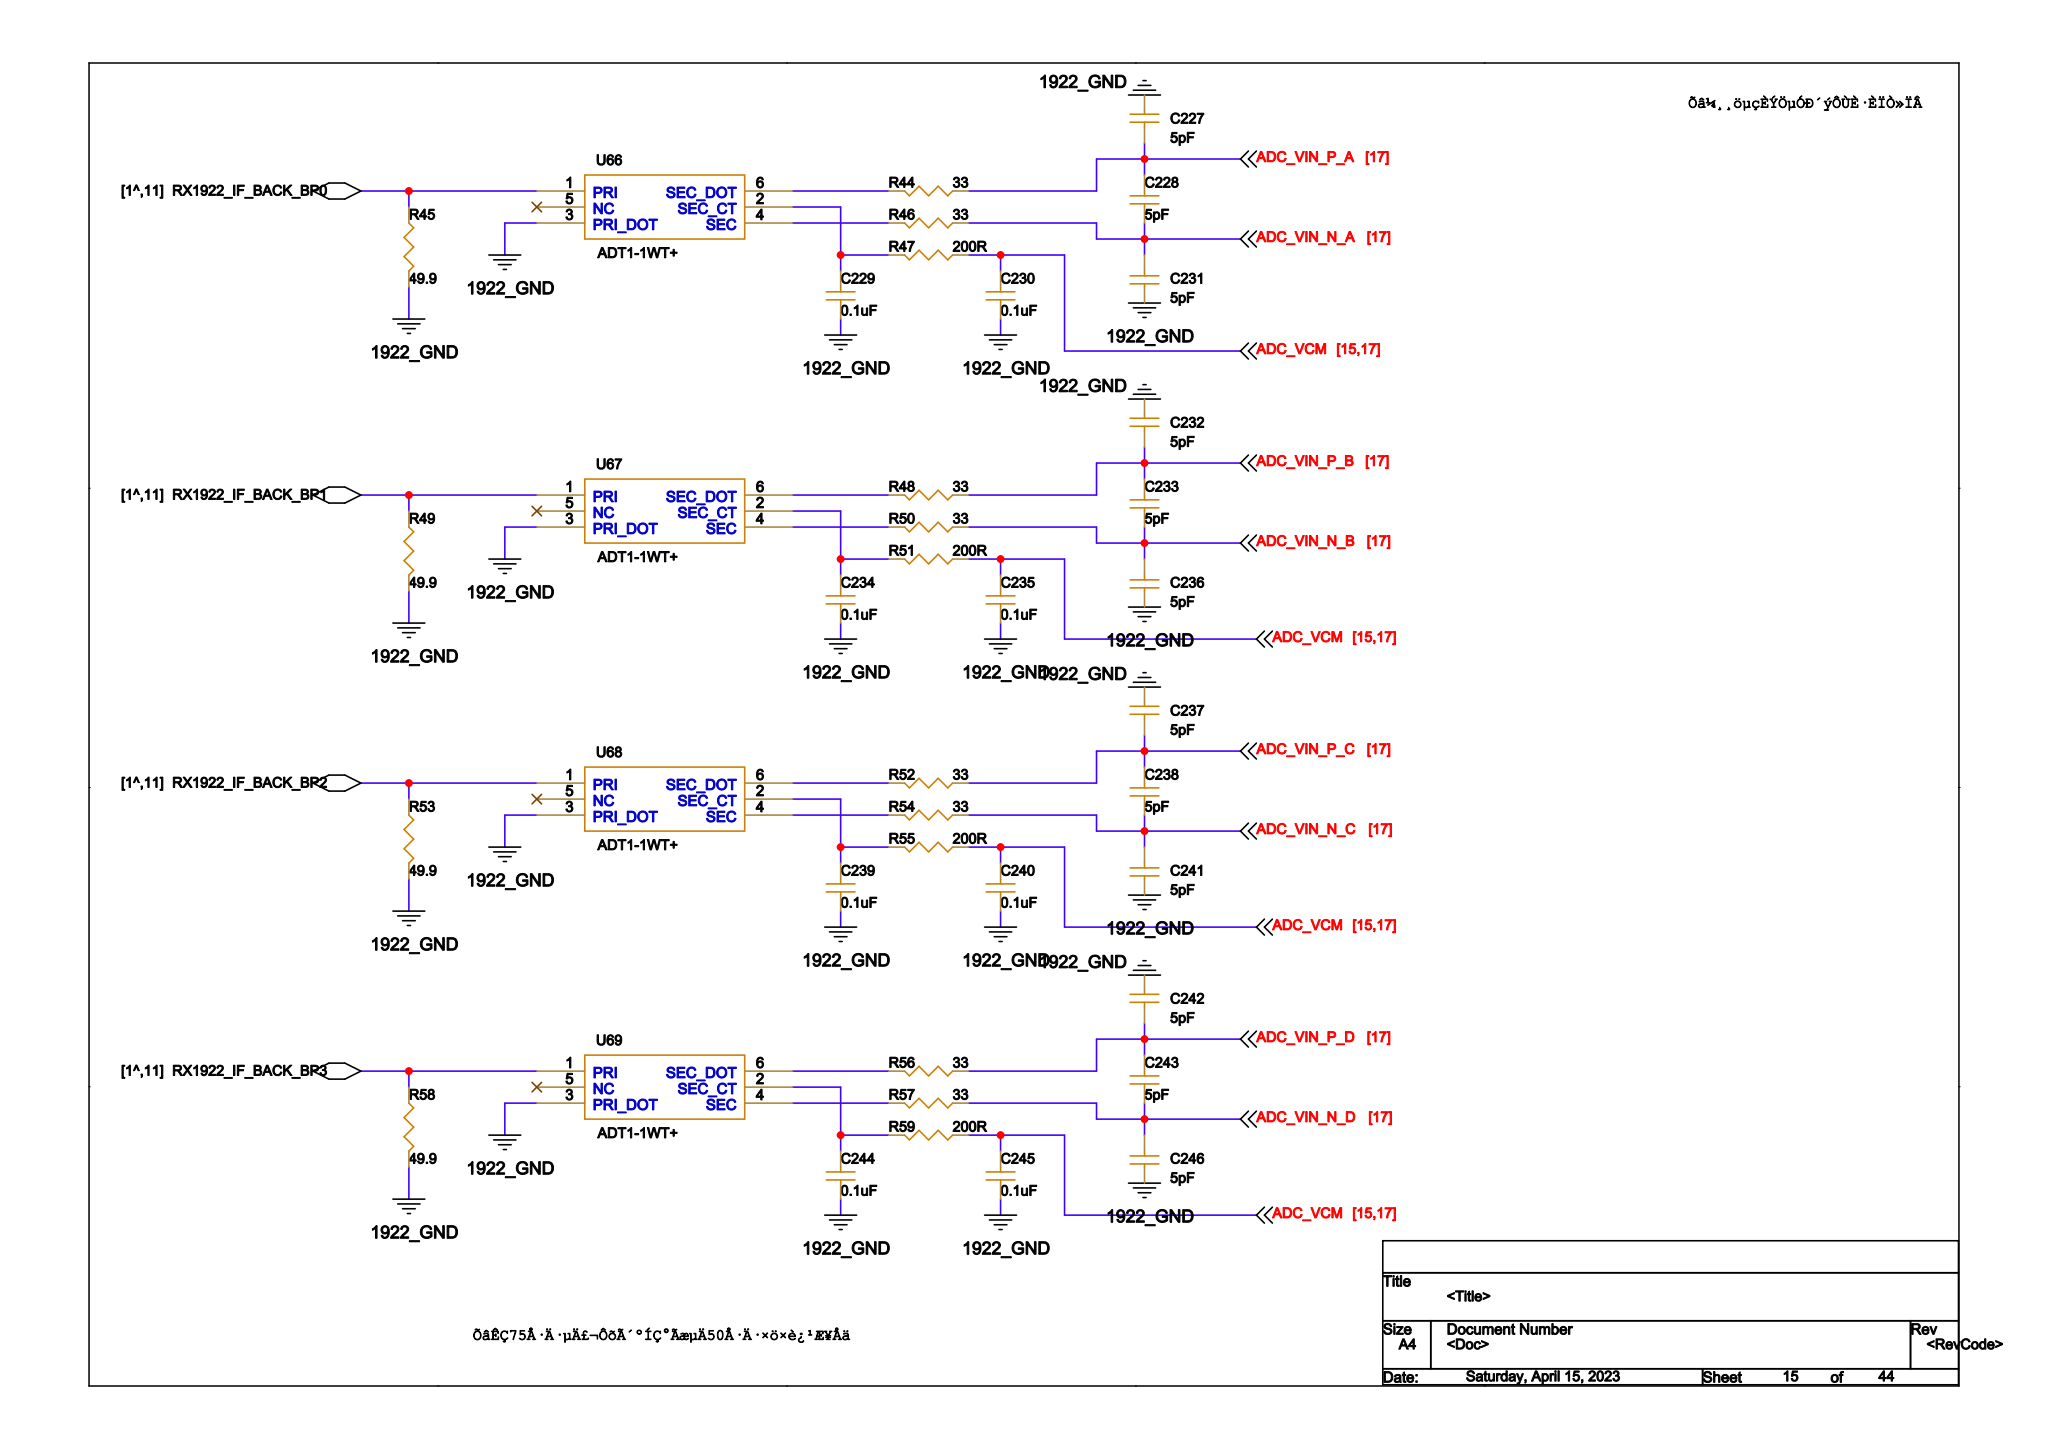Circuit board | Cadence Allegro | 1034 parts | 912 nets | one sheet of the schematic
Parts on this sheet (reference | value | footprint):
C227 | 5pF | C0402
C228 | 5pF | C0402
C229 | 0.1uF | C0402
C230 | 0.1uF | C0402
C231 | 5pF | C0402
C232 | 5pF | C0402
C233 | 5pF | C0402
C234 | 0.1uF | C0402
C235 | 0.1uF | C0402
C236 | 5pF | C0402
C237 | 5pF | C0402
C238 | 5pF | C0402
C239 | 0.1uF | C0402
C240 | 0.1uF | C0402
C241 | 5pF | C0402
C242 | 5pF | C0402
C243 | 5pF | C0402
C244 | 0.1uF | C0402
C245 | 0.1uF | C0402
C246 | 5pF | C0402
R44 | 33 | R0402
R45 | 49.9 | R0402
R46 | 33 | R0402
R47 | 200R | R0402
R48 | 33 | R0402
R49 | 49.9 | R0402
R50 | 33 | R0402
R51 | 200R | R0402
R52 | 33 | R0402
R53 | 49.9 | R0402
R54 | 33 | R0402
R55 | 200R | R0402
R56 | 33 | R0402
R57 | 33 | R0402
R58 | 49.9 | R0402
R59 | 200R | R0402
U66 | ADT1-1WT+ | ADT1_1WT_BL
U67 | ADT1-1WT+ | ADT1_1WT_BL
U68 | ADT1-1WT+ | ADT1_1WT_BL
U69 | ADT1-1WT+ | ADT1_1WT_BL
Nets of these parts (net: part-pin ...):
ADC_VCM_D4: C230-2 C235-2 C240-2 C245-2 R47-1 R51-1 R55-1 R59-1
ADC_VIN_P_A_D4: C227-2 C228-2 R44-1
ADC_VIN_P_B_D4: C232-2 C233-2 R48-1
ADC_VIN_P_C_D4: C237-2 C238-2 R52-1
ADC_VIN_P_D_D4: C242-2 C243-2 R56-1
ADC_VIN_N_A_D4: C228-1 C231-2 R46-1
ADC_VIN_N_B_D4: C233-1 C236-2 R50-1
ADC_VIN_N_C_D4: C238-1 C241-2 R54-1
ADC_VIN_N_D_D4: C243-1 C246-2 R57-1
1922_GND: C227-1 C229-1 C230-1 C231-1 C232-1 C234-1 C235-1 C236-1 C237-1 C239-1 C240-1 C241-1 C242-1 C244-1 C245-1 C246-1 R45-2 R49-2 R53-2 R58-2 U66-3 U67-3 U68-3 U69-3
N411903_D4: C229-2 R47-2 U66-2
N412844_D4: C234-2 R51-2 U67-2
N413577_D4: C239-2 R55-2 U68-2
N414339_D4: C244-2 R59-2 U69-2
N412892_D4: R50-2 U67-4
N413625_D4: R54-2 U68-4
N103792_D4: R44-2 U66-6
N103796_D4: R46-2 U66-4
N412820_D4: R48-2 U67-6
N413553_D4: R52-2 U68-6
N414315_D4: R56-2 U69-6
N414387_D4: R57-2 U69-4
N186408: R49-1 U67-1
N186410: R53-1 U68-1
N186406: R45-1 U66-1
N186412: R58-1 U69-1